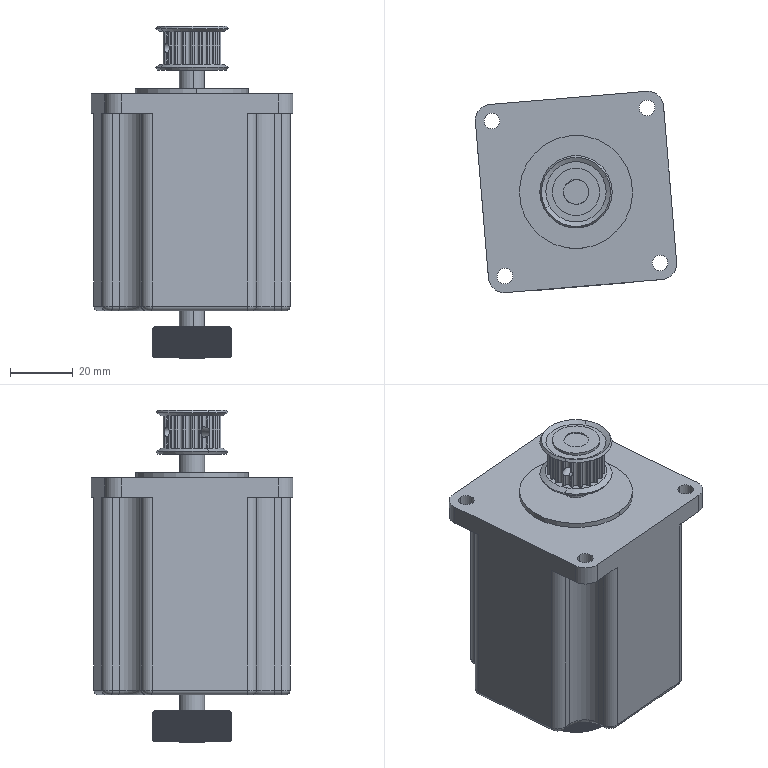Part | NX | features BREP 3 | 3 solids | 1388 faces | box 64.01 x 64.01 x 105.5 mm | volume 224733 mm3 | plane 776 | cylinder 581 | cone 19 | torus 12 | commonest cylinder face diameters 25 x371 1.02 x55 3.04 x46 1.7 x29 18.34 x24 3 x12